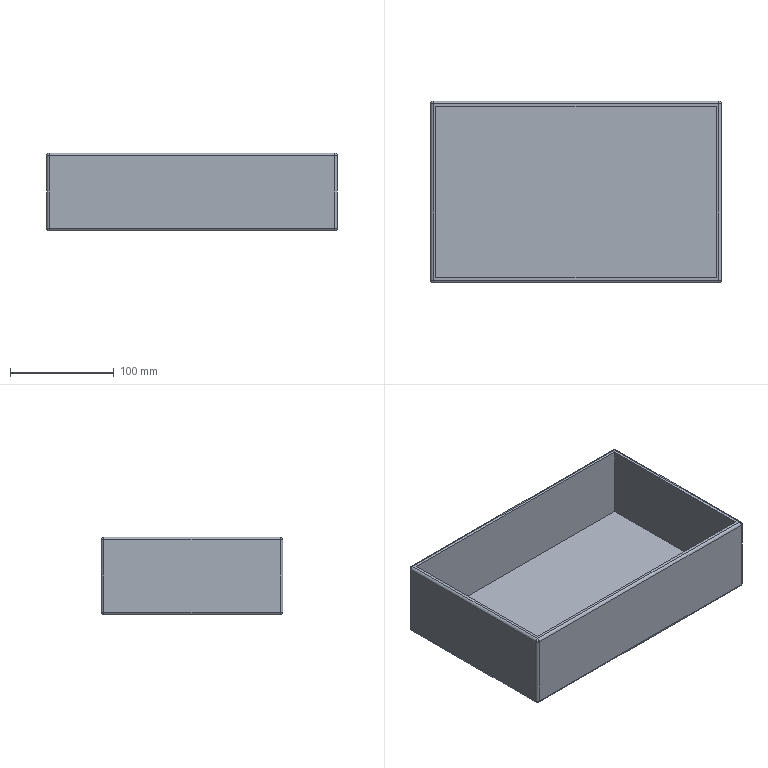Part | NX | features BREP 1 | 1 solid | 31 faces | box 280 x 175 x 75 mm | volume 553677 mm3 | cylinder 12 | plane 11 | sphere 8 | commonest cylinder face diameters 5 x12
STEP:
#1=CARTESIAN_POINT('',(277.5,172.5,75.));
#2=VERTEX_POINT('',#1);
#3=CARTESIAN_POINT('',(2.5,172.5,75.));
#4=VERTEX_POINT('',#3);
#5=CARTESIAN_POINT('',(0.,172.5,75.));
#6=DIRECTION('',(-1.,0.,0.));
#7=VECTOR('',#6,1000.);
#8=LINE('',#5,#7);
#9=EDGE_CURVE('',#2,#4,#8,.T.);
#10=ORIENTED_EDGE('',*,*,#9,.T.);
#11=CARTESIAN_POINT('',(2.5,2.5,75.));
#12=VERTEX_POINT('',#11);
#13=CARTESIAN_POINT('',(2.5,0.,75.));
#14=DIRECTION('',(0.,-1.,0.));
#15=VECTOR('',#14,1000.);
#16=LINE('',#13,#15);
#17=EDGE_CURVE('',#4,#12,#16,.T.);
#18=ORIENTED_EDGE('',*,*,#17,.T.);
#19=CARTESIAN_POINT('',(277.5,2.5,75.));
#20=VERTEX_POINT('',#19);
#21=CARTESIAN_POINT('',(0.,2.5,75.));
#22=DIRECTION('',(1.,0.,0.));
#23=VECTOR('',#22,1000.);
#24=LINE('',#21,#23);
#25=EDGE_CURVE('',#12,#20,#24,.T.);
#26=ORIENTED_EDGE('',*,*,#25,.T.);
#27=CARTESIAN_POINT('',(277.5,0.,75.));
#28=DIRECTION('',(0.,1.,0.));
#29=VECTOR('',#28,1000.);
#30=LINE('',#27,#29);
#31=EDGE_CURVE('',#20,#2,#30,.T.);
#32=ORIENTED_EDGE('',*,*,#31,.T.);
#33=EDGE_LOOP('',(#10,#18,#26,#32));
#34=FACE_BOUND('',#33,.T.);
#35=CARTESIAN_POINT('',(5.,170.,75.));
#36=VERTEX_POINT('',#35);
#37=CARTESIAN_POINT('',(5.,5.,75.));
#38=VERTEX_POINT('',#37);
#39=CARTESIAN_POINT('',(5.,0.,75.));
#40=DIRECTION('',(0.,-1.,0.));
#41=VECTOR('',#40,1000.);
#42=LINE('',#39,#41);
#43=EDGE_CURVE('',#36,#38,#42,.T.);
#44=ORIENTED_EDGE('',*,*,#43,.F.);
#45=CARTESIAN_POINT('',(275.,170.,75.));
#46=VERTEX_POINT('',#45);
#47=CARTESIAN_POINT('',(0.,170.,75.));
#48=DIRECTION('',(-1.,0.,0.));
#49=VECTOR('',#48,1000.);
#50=LINE('',#47,#49);
#51=EDGE_CURVE('',#46,#36,#50,.T.);
#52=ORIENTED_EDGE('',*,*,#51,.F.);
#53=CARTESIAN_POINT('',(275.,5.,75.));
#54=VERTEX_POINT('',#53);
#55=CARTESIAN_POINT('',(275.,0.,75.));
#56=DIRECTION('',(0.,1.,0.));
#57=VECTOR('',#56,1000.);
#58=LINE('',#55,#57);
#59=EDGE_CURVE('',#54,#46,#58,.T.);
#60=ORIENTED_EDGE('',*,*,#59,.F.);
#61=CARTESIAN_POINT('',(0.,5.,75.));
#62=DIRECTION('',(1.,0.,0.));
#63=VECTOR('',#62,1000.);
#64=LINE('',#61,#63);
#65=EDGE_CURVE('',#38,#54,#64,.T.);
#66=ORIENTED_EDGE('',*,*,#65,.F.);
#67=EDGE_LOOP('',(#44,#52,#60,#66));
#68=FACE_BOUND('',#67,.T.);
#69=CARTESIAN_POINT('',(0.,0.,75.));
#70=DIRECTION('',(0.,0.,-1.));
#71=DIRECTION('',(0.,-1.,0.));
#72=AXIS2_PLACEMENT_3D('',#69,#70,#71);
#73=PLANE('',#72);
#74=ADVANCED_FACE('',(#34,#68),#73,.F.);
#75=CARTESIAN_POINT('',(0.,2.5,72.5));
#76=VERTEX_POINT('',#75);
#77=CARTESIAN_POINT('',(0.,172.5,72.5));
#78=VERTEX_POINT('',#77);
#79=CARTESIAN_POINT('',(0.,0.,72.5));
#80=DIRECTION('',(0.,1.,0.));
#81=VECTOR('',#80,1000.);
#82=LINE('',#79,#81);
#83=EDGE_CURVE('',#76,#78,#82,.T.);
#84=ORIENTED_EDGE('',*,*,#83,.T.);
#85=CARTESIAN_POINT('',(0.,172.5,2.5));
#86=VERTEX_POINT('',#85);
#87=CARTESIAN_POINT('',(0.,172.5,75.));
#88=DIRECTION('',(0.,0.,-1.));
#89=VECTOR('',#88,1000.);
#90=LINE('',#87,#89);
#91=EDGE_CURVE('',#78,#86,#90,.T.);
#92=ORIENTED_EDGE('',*,*,#91,.T.);
#93=CARTESIAN_POINT('',(0.,2.5,2.5));
#94=VERTEX_POINT('',#93);
#95=CARTESIAN_POINT('',(0.,0.,2.5));
#96=DIRECTION('',(0.,-1.,0.));
#97=VECTOR('',#96,1000.);
#98=LINE('',#95,#97);
#99=EDGE_CURVE('',#86,#94,#98,.T.);
#100=ORIENTED_EDGE('',*,*,#99,.T.);
#101=CARTESIAN_POINT('',(0.,2.5,75.));
#102=DIRECTION('',(0.,0.,1.));
#103=VECTOR('',#102,1000.);
#104=LINE('',#101,#103);
#105=EDGE_CURVE('',#94,#76,#104,.T.);
#106=ORIENTED_EDGE('',*,*,#105,.T.);
#107=EDGE_LOOP('',(#84,#92,#100,#106));
#108=FACE_BOUND('',#107,.T.);
#109=CARTESIAN_POINT('',(0.,0.,75.));
#110=DIRECTION('',(1.,0.,0.));
#111=DIRECTION('',(0.,1.,0.));
#112=AXIS2_PLACEMENT_3D('',#109,#110,#111);
#113=PLANE('',#112);
#114=ADVANCED_FACE('',(#108),#113,.F.);
#115=CARTESIAN_POINT('',(277.5,0.,72.5));
#116=VERTEX_POINT('',#115);
#117=CARTESIAN_POINT('',(2.5,0.,72.5));
#118=VERTEX_POINT('',#117);
#119=CARTESIAN_POINT('',(0.,0.,72.5));
#120=DIRECTION('',(-1.,0.,0.));
#121=VECTOR('',#120,1000.);
#122=LINE('',#119,#121);
#123=EDGE_CURVE('',#116,#118,#122,.T.);
#124=ORIENTED_EDGE('',*,*,#123,.T.);
#125=CARTESIAN_POINT('',(2.5,0.,2.5));
#126=VERTEX_POINT('',#125);
#127=CARTESIAN_POINT('',(2.5,0.,75.));
#128=DIRECTION('',(0.,0.,-1.));
#129=VECTOR('',#128,1000.);
#130=LINE('',#127,#129);
#131=EDGE_CURVE('',#118,#126,#130,.T.);
#132=ORIENTED_EDGE('',*,*,#131,.T.);
#133=CARTESIAN_POINT('',(277.5,0.,2.5));
#134=VERTEX_POINT('',#133);
#135=CARTESIAN_POINT('',(280.,0.,2.5));
#136=DIRECTION('',(1.,0.,0.));
#137=VECTOR('',#136,1000.);
#138=LINE('',#135,#137);
#139=EDGE_CURVE('',#126,#134,#138,.T.);
#140=ORIENTED_EDGE('',*,*,#139,.T.);
#141=CARTESIAN_POINT('',(277.5,0.,75.));
#142=DIRECTION('',(0.,0.,1.));
#143=VECTOR('',#142,1000.);
#144=LINE('',#141,#143);
#145=EDGE_CURVE('',#134,#116,#144,.T.);
#146=ORIENTED_EDGE('',*,*,#145,.T.);
#147=EDGE_LOOP('',(#124,#132,#140,#146));
#148=FACE_BOUND('',#147,.T.);
#149=CARTESIAN_POINT('',(0.,0.,75.));
#150=DIRECTION('',(0.,1.,0.));
#151=DIRECTION('',(1.,0.,0.));
#152=AXIS2_PLACEMENT_3D('',#149,#150,#151);
#153=PLANE('',#152);
#154=ADVANCED_FACE('',(#148),#153,.F.);
#155=CARTESIAN_POINT('',(280.,172.5,2.5));
#156=VERTEX_POINT('',#155);
#157=CARTESIAN_POINT('',(280.,172.5,72.5));
#158=VERTEX_POINT('',#157);
#159=CARTESIAN_POINT('',(280.,172.5,75.));
#160=DIRECTION('',(0.,0.,1.));
#161=VECTOR('',#160,1000.);
#162=LINE('',#159,#161);
#163=EDGE_CURVE('',#156,#158,#162,.T.);
#164=ORIENTED_EDGE('',*,*,#163,.T.);
#165=CARTESIAN_POINT('',(280.,2.5,72.5));
#166=VERTEX_POINT('',#165);
#167=CARTESIAN_POINT('',(280.,0.,72.5));
#168=DIRECTION('',(0.,-1.,0.));
#169=VECTOR('',#168,1000.);
#170=LINE('',#167,#169);
#171=EDGE_CURVE('',#158,#166,#170,.T.);
#172=ORIENTED_EDGE('',*,*,#171,.T.);
#173=CARTESIAN_POINT('',(280.,2.5,2.5));
#174=VERTEX_POINT('',#173);
#175=CARTESIAN_POINT('',(280.,2.5,75.));
#176=DIRECTION('',(0.,0.,-1.));
#177=VECTOR('',#176,1000.);
#178=LINE('',#175,#177);
#179=EDGE_CURVE('',#166,#174,#178,.T.);
#180=ORIENTED_EDGE('',*,*,#179,.T.);
#181=CARTESIAN_POINT('',(280.,175.,2.5));
#182=DIRECTION('',(0.,1.,0.));
#183=VECTOR('',#182,1000.);
#184=LINE('',#181,#183);
#185=EDGE_CURVE('',#174,#156,#184,.T.);
#186=ORIENTED_EDGE('',*,*,#185,.T.);
#187=EDGE_LOOP('',(#164,#172,#180,#186));
#188=FACE_BOUND('',#187,.T.);
#189=CARTESIAN_POINT('',(280.,0.,75.));
#190=DIRECTION('',(-1.,0.,0.));
#191=DIRECTION('',(0.,0.,1.));
#192=AXIS2_PLACEMENT_3D('',#189,#190,#191);
#193=PLANE('',#192);
#194=ADVANCED_FACE('',(#188),#193,.F.);
#195=CARTESIAN_POINT('',(2.5,175.,2.5));
#196=VERTEX_POINT('',#195);
#197=CARTESIAN_POINT('',(2.5,175.,72.5));
#198=VERTEX_POINT('',#197);
#199=CARTESIAN_POINT('',(2.5,175.,75.));
#200=DIRECTION('',(0.,0.,1.));
#201=VECTOR('',#200,1000.);
#202=LINE('',#199,#201);
#203=EDGE_CURVE('',#196,#198,#202,.T.);
#204=ORIENTED_EDGE('',*,*,#203,.T.);
#205=CARTESIAN_POINT('',(277.5,175.,72.5));
#206=VERTEX_POINT('',#205);
#207=CARTESIAN_POINT('',(0.,175.,72.5));
#208=DIRECTION('',(1.,0.,0.));
#209=VECTOR('',#208,1000.);
#210=LINE('',#207,#209);
#211=EDGE_CURVE('',#198,#206,#210,.T.);
#212=ORIENTED_EDGE('',*,*,#211,.T.);
#213=CARTESIAN_POINT('',(277.5,175.,2.5));
#214=VERTEX_POINT('',#213);
#215=CARTESIAN_POINT('',(277.5,175.,75.));
#216=DIRECTION('',(0.,0.,-1.));
#217=VECTOR('',#216,1000.);
#218=LINE('',#215,#217);
#219=EDGE_CURVE('',#206,#214,#218,.T.);
#220=ORIENTED_EDGE('',*,*,#219,.T.);
#221=CARTESIAN_POINT('',(0.,175.,2.5));
#222=DIRECTION('',(-1.,0.,0.));
#223=VECTOR('',#222,1000.);
#224=LINE('',#221,#223);
#225=EDGE_CURVE('',#214,#196,#224,.T.);
#226=ORIENTED_EDGE('',*,*,#225,.T.);
#227=EDGE_LOOP('',(#204,#212,#220,#226));
#228=FACE_BOUND('',#227,.T.);
#229=CARTESIAN_POINT('',(0.,175.,75.));
#230=DIRECTION('',(0.,-1.,0.));
#231=DIRECTION('',(0.,0.,-1.));
#232=AXIS2_PLACEMENT_3D('',#229,#230,#231);
#233=PLANE('',#232);
#234=ADVANCED_FACE('',(#228),#233,.F.);
#235=CARTESIAN_POINT('',(277.5,2.5,0.));
#236=VERTEX_POINT('',#235);
#237=CARTESIAN_POINT('',(2.5,2.5,0.));
#238=VERTEX_POINT('',#237);
#239=CARTESIAN_POINT('',(0.,2.5,0.));
#240=DIRECTION('',(-1.,0.,0.));
#241=VECTOR('',#240,1000.);
#242=LINE('',#239,#241);
#243=EDGE_CURVE('',#236,#238,#242,.T.);
#244=ORIENTED_EDGE('',*,*,#243,.T.);
#245=CARTESIAN_POINT('',(2.5,172.5,0.));
#246=VERTEX_POINT('',#245);
#247=CARTESIAN_POINT('',(2.5,175.,0.));
#248=DIRECTION('',(0.,1.,0.));
#249=VECTOR('',#248,1000.);
#250=LINE('',#247,#249);
#251=EDGE_CURVE('',#238,#246,#250,.T.);
#252=ORIENTED_EDGE('',*,*,#251,.T.);
#253=CARTESIAN_POINT('',(277.5,172.5,0.));
#254=VERTEX_POINT('',#253);
#255=CARTESIAN_POINT('',(280.,172.5,0.));
#256=DIRECTION('',(1.,0.,0.));
#257=VECTOR('',#256,1000.);
#258=LINE('',#255,#257);
#259=EDGE_CURVE('',#246,#254,#258,.T.);
#260=ORIENTED_EDGE('',*,*,#259,.T.);
#261=CARTESIAN_POINT('',(277.5,0.,0.));
#262=DIRECTION('',(0.,-1.,0.));
#263=VECTOR('',#262,1000.);
#264=LINE('',#261,#263);
#265=EDGE_CURVE('',#254,#236,#264,.T.);
#266=ORIENTED_EDGE('',*,*,#265,.T.);
#267=EDGE_LOOP('',(#244,#252,#260,#266));
#268=FACE_BOUND('',#267,.T.);
#269=CARTESIAN_POINT('',(0.,0.,0.));
#270=DIRECTION('',(0.,0.,-1.));
#271=DIRECTION('',(0.,-1.,0.));
#272=AXIS2_PLACEMENT_3D('',#269,#270,#271);
#273=PLANE('',#272);
#274=ADVANCED_FACE('',(#268),#273,.T.);
#275=CARTESIAN_POINT('',(5.,170.,5.));
#276=VERTEX_POINT('',#275);
#277=CARTESIAN_POINT('',(5.,5.,5.));
#278=VERTEX_POINT('',#277);
#279=CARTESIAN_POINT('',(5.,0.,5.));
#280=DIRECTION('',(0.,-1.,0.));
#281=VECTOR('',#280,1000.);
#282=LINE('',#279,#281);
#283=EDGE_CURVE('',#276,#278,#282,.T.);
#284=ORIENTED_EDGE('',*,*,#283,.F.);
#285=CARTESIAN_POINT('',(5.,170.,75.));
#286=DIRECTION('',(0.,0.,-1.));
#287=VECTOR('',#286,1000.);
#288=LINE('',#285,#287);
#289=EDGE_CURVE('',#36,#276,#288,.T.);
#290=ORIENTED_EDGE('',*,*,#289,.F.);
#291=ORIENTED_EDGE('',*,*,#43,.T.);
#292=CARTESIAN_POINT('',(5.,5.,75.));
#293=DIRECTION('',(0.,0.,-1.));
#294=VECTOR('',#293,1000.);
#295=LINE('',#292,#294);
#296=EDGE_CURVE('',#38,#278,#295,.T.);
#297=ORIENTED_EDGE('',*,*,#296,.T.);
#298=EDGE_LOOP('',(#284,#290,#291,#297));
#299=FACE_BOUND('',#298,.T.);
#300=CARTESIAN_POINT('',(5.,0.,75.));
#301=DIRECTION('',(1.,0.,0.));
#302=DIRECTION('',(0.,1.,0.));
#303=AXIS2_PLACEMENT_3D('',#300,#301,#302);
#304=PLANE('',#303);
#305=ADVANCED_FACE('',(#299),#304,.T.);
#306=CARTESIAN_POINT('',(275.,5.,5.));
#307=VERTEX_POINT('',#306);
#308=CARTESIAN_POINT('',(0.,5.,5.));
#309=DIRECTION('',(1.,0.,0.));
#310=VECTOR('',#309,1000.);
#311=LINE('',#308,#310);
#312=EDGE_CURVE('',#278,#307,#311,.T.);
#313=ORIENTED_EDGE('',*,*,#312,.F.);
#314=ORIENTED_EDGE('',*,*,#296,.F.);
#315=ORIENTED_EDGE('',*,*,#65,.T.);
#316=CARTESIAN_POINT('',(275.,5.,75.));
#317=DIRECTION('',(0.,0.,-1.));
#318=VECTOR('',#317,1000.);
#319=LINE('',#316,#318);
#320=EDGE_CURVE('',#54,#307,#319,.T.);
#321=ORIENTED_EDGE('',*,*,#320,.T.);
#322=EDGE_LOOP('',(#313,#314,#315,#321));
#323=FACE_BOUND('',#322,.T.);
#324=CARTESIAN_POINT('',(0.,5.,75.));
#325=DIRECTION('',(0.,1.,0.));
#326=DIRECTION('',(1.,0.,0.));
#327=AXIS2_PLACEMENT_3D('',#324,#325,#326);
#328=PLANE('',#327);
#329=ADVANCED_FACE('',(#323),#328,.T.);
#330=CARTESIAN_POINT('',(275.,170.,5.));
#331=VERTEX_POINT('',#330);
#332=CARTESIAN_POINT('',(275.,0.,5.));
#333=DIRECTION('',(0.,1.,0.));
#334=VECTOR('',#333,1000.);
#335=LINE('',#332,#334);
#336=EDGE_CURVE('',#307,#331,#335,.T.);
#337=ORIENTED_EDGE('',*,*,#336,.F.);
#338=ORIENTED_EDGE('',*,*,#320,.F.);
#339=ORIENTED_EDGE('',*,*,#59,.T.);
#340=CARTESIAN_POINT('',(275.,170.,75.));
#341=DIRECTION('',(0.,0.,-1.));
#342=VECTOR('',#341,1000.);
#343=LINE('',#340,#342);
#344=EDGE_CURVE('',#46,#331,#343,.T.);
#345=ORIENTED_EDGE('',*,*,#344,.T.);
#346=EDGE_LOOP('',(#337,#338,#339,#345));
#347=FACE_BOUND('',#346,.T.);
#348=CARTESIAN_POINT('',(275.,0.,75.));
#349=DIRECTION('',(-1.,0.,0.));
#350=DIRECTION('',(0.,0.,1.));
#351=AXIS2_PLACEMENT_3D('',#348,#349,#350);
#352=PLANE('',#351);
#353=ADVANCED_FACE('',(#347),#352,.T.);
#354=CARTESIAN_POINT('',(0.,170.,5.));
#355=DIRECTION('',(-1.,0.,0.));
#356=VECTOR('',#355,1000.);
#357=LINE('',#354,#356);
#358=EDGE_CURVE('',#331,#276,#357,.T.);
#359=ORIENTED_EDGE('',*,*,#358,.F.);
#360=ORIENTED_EDGE('',*,*,#344,.F.);
#361=ORIENTED_EDGE('',*,*,#51,.T.);
#362=ORIENTED_EDGE('',*,*,#289,.T.);
#363=EDGE_LOOP('',(#359,#360,#361,#362));
#364=FACE_BOUND('',#363,.T.);
#365=CARTESIAN_POINT('',(0.,170.,75.));
#366=DIRECTION('',(0.,-1.,0.));
#367=DIRECTION('',(0.,0.,-1.));
#368=AXIS2_PLACEMENT_3D('',#365,#366,#367);
#369=PLANE('',#368);
#370=ADVANCED_FACE('',(#364),#369,.T.);
#371=ORIENTED_EDGE('',*,*,#283,.T.);
#372=ORIENTED_EDGE('',*,*,#312,.T.);
#373=ORIENTED_EDGE('',*,*,#336,.T.);
#374=ORIENTED_EDGE('',*,*,#358,.T.);
#375=EDGE_LOOP('',(#371,#372,#373,#374));
#376=FACE_BOUND('',#375,.T.);
#377=CARTESIAN_POINT('',(0.,0.,5.));
#378=DIRECTION('',(0.,0.,-1.));
#379=DIRECTION('',(0.,-1.,0.));
#380=AXIS2_PLACEMENT_3D('',#377,#378,#379);
#381=PLANE('',#380);
#382=ADVANCED_FACE('',(#376),#381,.F.);
#383=CARTESIAN_POINT('',(277.5,172.5,2.5));
#384=DIRECTION('',(0.,1.,0.));
#385=DIRECTION('',(0.,0.,1.));
#386=AXIS2_PLACEMENT_3D('',#383,#384,#385);
#387=CIRCLE('',#386,2.5);
#388=EDGE_CURVE('',#156,#254,#387,.T.);
#389=ORIENTED_EDGE('',*,*,#388,.F.);
#390=ORIENTED_EDGE('',*,*,#185,.F.);
#391=CARTESIAN_POINT('',(277.5,2.5,2.5));
#392=DIRECTION('',(0.,-1.,0.));
#393=DIRECTION('',(0.,0.,-1.));
#394=AXIS2_PLACEMENT_3D('',#391,#392,#393);
#395=CIRCLE('',#394,2.5);
#396=EDGE_CURVE('',#236,#174,#395,.T.);
#397=ORIENTED_EDGE('',*,*,#396,.F.);
#398=ORIENTED_EDGE('',*,*,#265,.F.);
#399=EDGE_LOOP('',(#389,#390,#397,#398));
#400=FACE_BOUND('',#399,.T.);
#401=CARTESIAN_POINT('',(277.5,0.,2.5));
#402=DIRECTION('',(0.,-1.,0.));
#403=DIRECTION('',(0.,0.,-1.));
#404=AXIS2_PLACEMENT_3D('',#401,#402,#403);
#405=CYLINDRICAL_SURFACE('',#404,2.5);
#406=ADVANCED_FACE('',(#400),#405,.T.);
#407=CARTESIAN_POINT('',(277.5,172.5,2.5));
#408=DIRECTION('',(0.,0.,1.));
#409=DIRECTION('',(-1.,0.,0.));
#410=AXIS2_PLACEMENT_3D('',#407,#408,#409);
#411=CIRCLE('',#410,2.5);
#412=EDGE_CURVE('',#156,#214,#411,.T.);
#413=ORIENTED_EDGE('',*,*,#412,.F.);
#414=ORIENTED_EDGE('',*,*,#388,.T.);
#415=CARTESIAN_POINT('',(277.5,172.5,2.5));
#416=DIRECTION('',(-1.,0.,0.));
#417=DIRECTION('',(0.,0.,-1.));
#418=AXIS2_PLACEMENT_3D('',#415,#416,#417);
#419=CIRCLE('',#418,2.5);
#420=EDGE_CURVE('',#214,#254,#419,.T.);
#421=ORIENTED_EDGE('',*,*,#420,.F.);
#422=EDGE_LOOP('',(#413,#414,#421));
#423=FACE_BOUND('',#422,.T.);
#424=CARTESIAN_POINT('',(277.5,172.5,2.5));
#425=DIRECTION('',(0.,0.,-1.));
#426=DIRECTION('',(1.,0.,0.));
#427=AXIS2_PLACEMENT_3D('',#424,#425,#426);
#428=SPHERICAL_SURFACE('',#427,2.5);
#429=ADVANCED_FACE('',(#423),#428,.T.);
#430=CARTESIAN_POINT('',(277.5,2.5,2.5));
#431=DIRECTION('',(-1.,0.,0.));
#432=DIRECTION('',(0.,0.,-1.));
#433=AXIS2_PLACEMENT_3D('',#430,#431,#432);
#434=CIRCLE('',#433,2.5);
#435=EDGE_CURVE('',#236,#134,#434,.T.);
#436=ORIENTED_EDGE('',*,*,#435,.F.);
#437=ORIENTED_EDGE('',*,*,#396,.T.);
#438=CARTESIAN_POINT('',(277.5,2.5,2.5));
#439=DIRECTION('',(0.,0.,1.));
#440=DIRECTION('',(-1.,0.,0.));
#441=AXIS2_PLACEMENT_3D('',#438,#439,#440);
#442=CIRCLE('',#441,2.5);
#443=EDGE_CURVE('',#134,#174,#442,.T.);
#444=ORIENTED_EDGE('',*,*,#443,.F.);
#445=EDGE_LOOP('',(#436,#437,#444));
#446=FACE_BOUND('',#445,.T.);
#447=CARTESIAN_POINT('',(277.5,2.5,2.5));
#448=DIRECTION('',(0.,0.,-1.));
#449=DIRECTION('',(1.,0.,0.));
#450=AXIS2_PLACEMENT_3D('',#447,#448,#449);
#451=SPHERICAL_SURFACE('',#450,2.5);
#452=ADVANCED_FACE('',(#446),#451,.T.);
#453=ORIENTED_EDGE('',*,*,#420,.T.);
#454=ORIENTED_EDGE('',*,*,#259,.F.);
#455=CARTESIAN_POINT('',(2.5,172.5,2.5));
#456=DIRECTION('',(-1.,0.,0.));
#457=DIRECTION('',(0.,0.,1.));
#458=AXIS2_PLACEMENT_3D('',#455,#456,#457);
#459=CIRCLE('',#458,2.5);
#460=EDGE_CURVE('',#196,#246,#459,.T.);
#461=ORIENTED_EDGE('',*,*,#460,.F.);
#462=ORIENTED_EDGE('',*,*,#225,.F.);
#463=EDGE_LOOP('',(#453,#454,#461,#462));
#464=FACE_BOUND('',#463,.T.);
#465=CARTESIAN_POINT('',(0.,172.5,2.5));
#466=DIRECTION('',(1.,0.,0.));
#467=DIRECTION('',(0.,0.,-1.));
#468=AXIS2_PLACEMENT_3D('',#465,#466,#467);
#469=CYLINDRICAL_SURFACE('',#468,2.5);
#470=ADVANCED_FACE('',(#464),#469,.T.);
#471=ORIENTED_EDGE('',*,*,#412,.T.);
#472=ORIENTED_EDGE('',*,*,#219,.F.);
#473=CARTESIAN_POINT('',(277.5,172.5,72.5));
#474=DIRECTION('',(0.,0.,1.));
#475=DIRECTION('',(1.,0.,0.));
#476=AXIS2_PLACEMENT_3D('',#473,#474,#475);
#477=CIRCLE('',#476,2.5);
#478=EDGE_CURVE('',#158,#206,#477,.T.);
#479=ORIENTED_EDGE('',*,*,#478,.F.);
#480=ORIENTED_EDGE('',*,*,#163,.F.);
#481=EDGE_LOOP('',(#471,#472,#479,#480));
#482=FACE_BOUND('',#481,.T.);
#483=CARTESIAN_POINT('',(277.5,172.5,75.));
#484=DIRECTION('',(0.,0.,-1.));
#485=DIRECTION('',(-1.,0.,0.));
#486=AXIS2_PLACEMENT_3D('',#483,#484,#485);
#487=CYLINDRICAL_SURFACE('',#486,2.5);
#488=ADVANCED_FACE('',(#482),#487,.T.);
#489=CARTESIAN_POINT('',(277.5,2.5,72.5));
#490=DIRECTION('',(0.,-1.,0.));
#491=DIRECTION('',(0.,0.,-1.));
#492=AXIS2_PLACEMENT_3D('',#489,#490,#491);
#493=CIRCLE('',#492,2.5);
#494=EDGE_CURVE('',#166,#20,#493,.T.);
#495=ORIENTED_EDGE('',*,*,#494,.F.);
#496=ORIENTED_EDGE('',*,*,#171,.F.);
#497=CARTESIAN_POINT('',(277.5,172.5,72.5));
#498=DIRECTION('',(0.,1.,0.));
#499=DIRECTION('',(0.,0.,1.));
#500=AXIS2_PLACEMENT_3D('',#497,#498,#499);
#501=CIRCLE('',#500,2.5);
#502=EDGE_CURVE('',#2,#158,#501,.T.);
#503=ORIENTED_EDGE('',*,*,#502,.F.);
#504=ORIENTED_EDGE('',*,*,#31,.F.);
#505=EDGE_LOOP('',(#495,#496,#503,#504));
#506=FACE_BOUND('',#505,.T.);
#507=CARTESIAN_POINT('',(277.5,0.,72.5));
#508=DIRECTION('',(0.,1.,0.));
#509=DIRECTION('',(0.,0.,1.));
#510=AXIS2_PLACEMENT_3D('',#507,#508,#509);
#511=CYLINDRICAL_SURFACE('',#510,2.5);
#512=ADVANCED_FACE('',(#506),#511,.T.);
#513=ORIENTED_EDGE('',*,*,#443,.T.);
#514=ORIENTED_EDGE('',*,*,#179,.F.);
#515=CARTESIAN_POINT('',(277.5,2.5,72.5));
#516=DIRECTION('',(0.,0.,1.));
#517=DIRECTION('',(1.,0.,0.));
#518=AXIS2_PLACEMENT_3D('',#515,#516,#517);
#519=CIRCLE('',#518,2.5);
#520=EDGE_CURVE('',#116,#166,#519,.T.);
#521=ORIENTED_EDGE('',*,*,#520,.F.);
#522=ORIENTED_EDGE('',*,*,#145,.F.);
#523=EDGE_LOOP('',(#513,#514,#521,#522));
#524=FACE_BOUND('',#523,.T.);
#525=CARTESIAN_POINT('',(277.5,2.5,75.));
#526=DIRECTION('',(0.,0.,-1.));
#527=DIRECTION('',(-1.,0.,0.));
#528=AXIS2_PLACEMENT_3D('',#525,#526,#527);
#529=CYLINDRICAL_SURFACE('',#528,2.5);
#530=ADVANCED_FACE('',(#524),#529,.T.);
#531=ORIENTED_EDGE('',*,*,#435,.T.);
#532=ORIENTED_EDGE('',*,*,#139,.F.);
#533=CARTESIAN_POINT('',(2.5,2.5,2.5));
#534=DIRECTION('',(-1.,0.,0.));
#535=DIRECTION('',(0.,0.,1.));
#536=AXIS2_PLACEMENT_3D('',#533,#534,#535);
#537=CIRCLE('',#536,2.5);
#538=EDGE_CURVE('',#238,#126,#537,.T.);
#539=ORIENTED_EDGE('',*,*,#538,.F.);
#540=ORIENTED_EDGE('',*,*,#243,.F.);
#541=EDGE_LOOP('',(#531,#532,#539,#540));
#542=FACE_BOUND('',#541,.T.);
#543=CARTESIAN_POINT('',(0.,2.5,2.5));
#544=DIRECTION('',(-1.,0.,0.));
#545=DIRECTION('',(0.,0.,1.));
#546=AXIS2_PLACEMENT_3D('',#543,#544,#545);
#547=CYLINDRICAL_SURFACE('',#546,2.5);
#548=ADVANCED_FACE('',(#542),#547,.T.);
#549=CARTESIAN_POINT('',(2.5,172.5,2.5));
#550=DIRECTION('',(0.,1.,0.));
#551=DIRECTION('',(0.,0.,1.));
#552=AXIS2_PLACEMENT_3D('',#549,#550,#551);
#553=CIRCLE('',#552,2.5);
#554=EDGE_CURVE('',#246,#86,#553,.T.);
#555=ORIENTED_EDGE('',*,*,#554,.F.);
#556=ORIENTED_EDGE('',*,*,#251,.F.);
#557=CARTESIAN_POINT('',(2.5,2.5,2.5));
#558=DIRECTION('',(0.,-1.,0.));
#559=DIRECTION('',(0.,0.,-1.));
#560=AXIS2_PLACEMENT_3D('',#557,#558,#559);
#561=CIRCLE('',#560,2.5);
#562=EDGE_CURVE('',#94,#238,#561,.T.);
#563=ORIENTED_EDGE('',*,*,#562,.F.);
#564=ORIENTED_EDGE('',*,*,#99,.F.);
#565=EDGE_LOOP('',(#555,#556,#563,#564));
#566=FACE_BOUND('',#565,.T.);
#567=CARTESIAN_POINT('',(2.5,0.,2.5));
#568=DIRECTION('',(0.,1.,0.));
#569=DIRECTION('',(0.,0.,1.));
#570=AXIS2_PLACEMENT_3D('',#567,#568,#569);
#571=CYLINDRICAL_SURFACE('',#570,2.5);
#572=ADVANCED_FACE('',(#566),#571,.T.);
#573=ORIENTED_EDGE('',*,*,#460,.T.);
#574=ORIENTED_EDGE('',*,*,#554,.T.);
#575=CARTESIAN_POINT('',(2.5,172.5,2.5));
#576=DIRECTION('',(0.,0.,1.));
#577=DIRECTION('',(-1.,0.,0.));
#578=AXIS2_PLACEMENT_3D('',#575,#576,#577);
#579=CIRCLE('',#578,2.5);
#580=EDGE_CURVE('',#196,#86,#579,.T.);
#581=ORIENTED_EDGE('',*,*,#580,.F.);
#582=EDGE_LOOP('',(#573,#574,#581));
#583=FACE_BOUND('',#582,.T.);
#584=CARTESIAN_POINT('',(2.5,172.5,2.5));
#585=DIRECTION('',(0.,0.,-1.));
#586=DIRECTION('',(1.,0.,0.));
#587=AXIS2_PLACEMENT_3D('',#584,#585,#586);
#588=SPHERICAL_SURFACE('',#587,2.5);
#589=ADVANCED_FACE('',(#583),#588,.T.);
#590=ORIENTED_EDGE('',*,*,#502,.T.);
#591=ORIENTED_EDGE('',*,*,#478,.T.);
#592=CARTESIAN_POINT('',(277.5,172.5,72.5));
#593=DIRECTION('',(-1.,0.,0.));
#594=DIRECTION('',(0.,0.,-1.));
#595=AXIS2_PLACEMENT_3D('',#592,#593,#594);
#596=CIRCLE('',#595,2.5);
#597=EDGE_CURVE('',#2,#206,#596,.T.);
#598=ORIENTED_EDGE('',*,*,#597,.F.);
#599=EDGE_LOOP('',(#590,#591,#598));
#600=FACE_BOUND('',#599,.T.);
#601=CARTESIAN_POINT('',(277.5,172.5,72.5));
#602=DIRECTION('',(0.,0.,-1.));
#603=DIRECTION('',(1.,0.,0.));
#604=AXIS2_PLACEMENT_3D('',#601,#602,#603);
#605=SPHERICAL_SURFACE('',#604,2.5);
#606=ADVANCED_FACE('',(#600),#605,.T.);
#607=ORIENTED_EDGE('',*,*,#520,.T.);
#608=ORIENTED_EDGE('',*,*,#494,.T.);
#609=CARTESIAN_POINT('',(277.5,2.5,72.5));
#610=DIRECTION('',(-1.,0.,0.));
#611=DIRECTION('',(0.,0.,-1.));
#612=AXIS2_PLACEMENT_3D('',#609,#610,#611);
#613=CIRCLE('',#612,2.5);
#614=EDGE_CURVE('',#116,#20,#613,.T.);
#615=ORIENTED_EDGE('',*,*,#614,.F.);
#616=EDGE_LOOP('',(#607,#608,#615));
#617=FACE_BOUND('',#616,.T.);
#618=CARTESIAN_POINT('',(277.5,2.5,72.5));
#619=DIRECTION('',(0.,0.,-1.));
#620=DIRECTION('',(1.,0.,0.));
#621=AXIS2_PLACEMENT_3D('',#618,#619,#620);
#622=SPHERICAL_SURFACE('',#621,2.5);
#623=ADVANCED_FACE('',(#617),#622,.T.);
#624=ORIENTED_EDGE('',*,*,#562,.T.);
#625=ORIENTED_EDGE('',*,*,#538,.T.);
#626=CARTESIAN_POINT('',(2.5,2.5,2.5));
#627=DIRECTION('',(0.,0.,1.));
#628=DIRECTION('',(-1.,0.,0.));
#629=AXIS2_PLACEMENT_3D('',#626,#627,#628);
#630=CIRCLE('',#629,2.5);
#631=EDGE_CURVE('',#94,#126,#630,.T.);
#632=ORIENTED_EDGE('',*,*,#631,.F.);
#633=EDGE_LOOP('',(#624,#625,#632));
#634=FACE_BOUND('',#633,.T.);
#635=CARTESIAN_POINT('',(2.5,2.5,2.5));
#636=DIRECTION('',(0.,0.,-1.));
#637=DIRECTION('',(1.,0.,0.));
#638=AXIS2_PLACEMENT_3D('',#635,#636,#637);
#639=SPHERICAL_SURFACE('',#638,2.5);
#640=ADVANCED_FACE('',(#634),#639,.T.);
#641=ORIENTED_EDGE('',*,*,#580,.T.);
#642=ORIENTED_EDGE('',*,*,#91,.F.);
#643=CARTESIAN_POINT('',(2.5,172.5,72.5));
#644=DIRECTION('',(0.,0.,1.));
#645=DIRECTION('',(1.,0.,0.));
#646=AXIS2_PLACEMENT_3D('',#643,#644,#645);
#647=CIRCLE('',#646,2.5);
#648=EDGE_CURVE('',#198,#78,#647,.T.);
#649=ORIENTED_EDGE('',*,*,#648,.F.);
#650=ORIENTED_EDGE('',*,*,#203,.F.);
#651=EDGE_LOOP('',(#641,#642,#649,#650));
#652=FACE_BOUND('',#651,.T.);
#653=CARTESIAN_POINT('',(2.5,172.5,75.));
#654=DIRECTION('',(0.,0.,-1.));
#655=DIRECTION('',(-1.,0.,0.));
#656=AXIS2_PLACEMENT_3D('',#653,#654,#655);
#657=CYLINDRICAL_SURFACE('',#656,2.5);
#658=ADVANCED_FACE('',(#652),#657,.T.);
#659=ORIENTED_EDGE('',*,*,#597,.T.);
#660=ORIENTED_EDGE('',*,*,#211,.F.);
#661=CARTESIAN_POINT('',(2.5,172.5,72.5));
#662=DIRECTION('',(-1.,0.,0.));
#663=DIRECTION('',(0.,0.,1.));
#664=AXIS2_PLACEMENT_3D('',#661,#662,#663);
#665=CIRCLE('',#664,2.5);
#666=EDGE_CURVE('',#4,#198,#665,.T.);
#667=ORIENTED_EDGE('',*,*,#666,.F.);
#668=ORIENTED_EDGE('',*,*,#9,.F.);
#669=EDGE_LOOP('',(#659,#660,#667,#668));
#670=FACE_BOUND('',#669,.T.);
#671=CARTESIAN_POINT('',(0.,172.5,72.5));
#672=DIRECTION('',(-1.,0.,0.));
#673=DIRECTION('',(0.,0.,1.));
#674=AXIS2_PLACEMENT_3D('',#671,#672,#673);
#675=CYLINDRICAL_SURFACE('',#674,2.5);
#676=ADVANCED_FACE('',(#670),#675,.T.);
#677=ORIENTED_EDGE('',*,*,#614,.T.);
#678=ORIENTED_EDGE('',*,*,#25,.F.);
#679=CARTESIAN_POINT('',(2.5,2.5,72.5));
#680=DIRECTION('',(-1.,0.,0.));
#681=DIRECTION('',(0.,0.,1.));
#682=AXIS2_PLACEMENT_3D('',#679,#680,#681);
#683=CIRCLE('',#682,2.5);
#684=EDGE_CURVE('',#118,#12,#683,.T.);
#685=ORIENTED_EDGE('',*,*,#684,.F.);
#686=ORIENTED_EDGE('',*,*,#123,.F.);
#687=EDGE_LOOP('',(#677,#678,#685,#686));
#688=FACE_BOUND('',#687,.T.);
#689=CARTESIAN_POINT('',(0.,2.5,72.5));
#690=DIRECTION('',(1.,0.,0.));
#691=DIRECTION('',(0.,0.,-1.));
#692=AXIS2_PLACEMENT_3D('',#689,#690,#691);
#693=CYLINDRICAL_SURFACE('',#692,2.5);
#694=ADVANCED_FACE('',(#688),#693,.T.);
#695=ORIENTED_EDGE('',*,*,#631,.T.);
#696=ORIENTED_EDGE('',*,*,#131,.F.);
#697=CARTESIAN_POINT('',(2.5,2.5,72.5));
#698=DIRECTION('',(0.,0.,1.));
#699=DIRECTION('',(1.,0.,0.));
#700=AXIS2_PLACEMENT_3D('',#697,#698,#699);
#701=CIRCLE('',#700,2.5);
#702=EDGE_CURVE('',#76,#118,#701,.T.);
#703=ORIENTED_EDGE('',*,*,#702,.F.);
#704=ORIENTED_EDGE('',*,*,#105,.F.);
#705=EDGE_LOOP('',(#695,#696,#703,#704));
#706=FACE_BOUND('',#705,.T.);
#707=CARTESIAN_POINT('',(2.5,2.5,75.));
#708=DIRECTION('',(0.,0.,-1.));
#709=DIRECTION('',(-1.,0.,0.));
#710=AXIS2_PLACEMENT_3D('',#707,#708,#709);
#711=CYLINDRICAL_SURFACE('',#710,2.5);
#712=ADVANCED_FACE('',(#706),#711,.T.);
#713=ORIENTED_EDGE('',*,*,#666,.T.);
#714=ORIENTED_EDGE('',*,*,#648,.T.);
#715=CARTESIAN_POINT('',(2.5,172.5,72.5));
#716=DIRECTION('',(0.,-1.,0.));
#717=DIRECTION('',(0.,0.,1.));
#718=AXIS2_PLACEMENT_3D('',#715,#716,#717);
#719=CIRCLE('',#718,2.5);
#720=EDGE_CURVE('',#4,#78,#719,.T.);
#721=ORIENTED_EDGE('',*,*,#720,.F.);
#722=EDGE_LOOP('',(#713,#714,#721));
#723=FACE_BOUND('',#722,.T.);
#724=CARTESIAN_POINT('',(2.5,172.5,72.5));
#725=DIRECTION('',(0.,0.,-1.));
#726=DIRECTION('',(1.,0.,0.));
#727=AXIS2_PLACEMENT_3D('',#724,#725,#726);
#728=SPHERICAL_SURFACE('',#727,2.5);
#729=ADVANCED_FACE('',(#723),#728,.T.);
#730=ORIENTED_EDGE('',*,*,#702,.T.);
#731=ORIENTED_EDGE('',*,*,#684,.T.);
#732=CARTESIAN_POINT('',(2.5,2.5,72.5));
#733=DIRECTION('',(0.,1.,0.));
#734=DIRECTION('',(0.,0.,-1.));
#735=AXIS2_PLACEMENT_3D('',#732,#733,#734);
#736=CIRCLE('',#735,2.5);
#737=EDGE_CURVE('',#76,#12,#736,.T.);
#738=ORIENTED_EDGE('',*,*,#737,.F.);
#739=EDGE_LOOP('',(#730,#731,#738));
#740=FACE_BOUND('',#739,.T.);
#741=CARTESIAN_POINT('',(2.5,2.5,72.5));
#742=DIRECTION('',(0.,0.,-1.));
#743=DIRECTION('',(1.,0.,0.));
#744=AXIS2_PLACEMENT_3D('',#741,#742,#743);
#745=SPHERICAL_SURFACE('',#744,2.5);
#746=ADVANCED_FACE('',(#740),#745,.T.);
#747=ORIENTED_EDGE('',*,*,#720,.T.);
#748=ORIENTED_EDGE('',*,*,#83,.F.);
#749=ORIENTED_EDGE('',*,*,#737,.T.);
#750=ORIENTED_EDGE('',*,*,#17,.F.);
#751=EDGE_LOOP('',(#747,#748,#749,#750));
#752=FACE_BOUND('',#751,.T.);
#753=CARTESIAN_POINT('',(2.5,0.,72.5));
#754=DIRECTION('',(0.,-1.,0.));
#755=DIRECTION('',(0.,0.,-1.));
#756=AXIS2_PLACEMENT_3D('',#753,#754,#755);
#757=CYLINDRICAL_SURFACE('',#756,2.5);
#758=ADVANCED_FACE('',(#752),#757,.T.);
#759=CLOSED_SHELL('',(#74,#114,#154,#194,#234,#274,#305,#329,#353,#370,#382,#406,#429,#452,#470,#488,#512,#530,#548,#572,#589,#606,#623,#640,#658,#676,#694,#712,#729,#746,#758));
#760=MANIFOLD_SOLID_BREP('',#759);
#761=(LENGTH_UNIT()NAMED_UNIT(*)SI_UNIT(.MILLI.,.METRE.));
#762=UNCERTAINTY_MEASURE_WITH_UNIT(LENGTH_MEASURE(0.00001),#761,'','');
#763=(NAMED_UNIT(*)PLANE_ANGLE_UNIT()SI_UNIT($,.RADIAN.));
#764=(NAMED_UNIT(*)SI_UNIT($,.STERADIAN.)SOLID_ANGLE_UNIT());
#765=(GEOMETRIC_REPRESENTATION_CONTEXT(3)GLOBAL_UNCERTAINTY_ASSIGNED_CONTEXT((#762))GLOBAL_UNIT_ASSIGNED_CONTEXT((#761,#763,#764))REPRESENTATION_CONTEXT('',''));
#766=ADVANCED_BREP_SHAPE_REPRESENTATION('',(#760),#765);